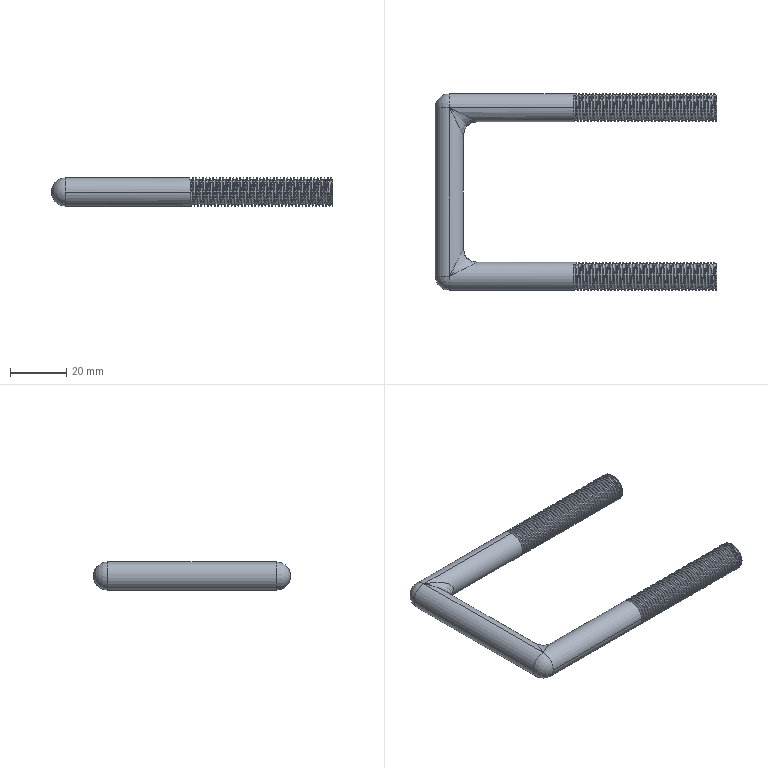Part | SolidWorks | features Helix 2, SweepCut 2, Fillet 1, Sweep 1 | 1 solid | 184 faces | box 100 x 70 x 10 mm | volume 18547 mm3 | cylinder 172 | spline 6 | plane 4 | sphere 2 | commonest cylinder face diameters 10 x172